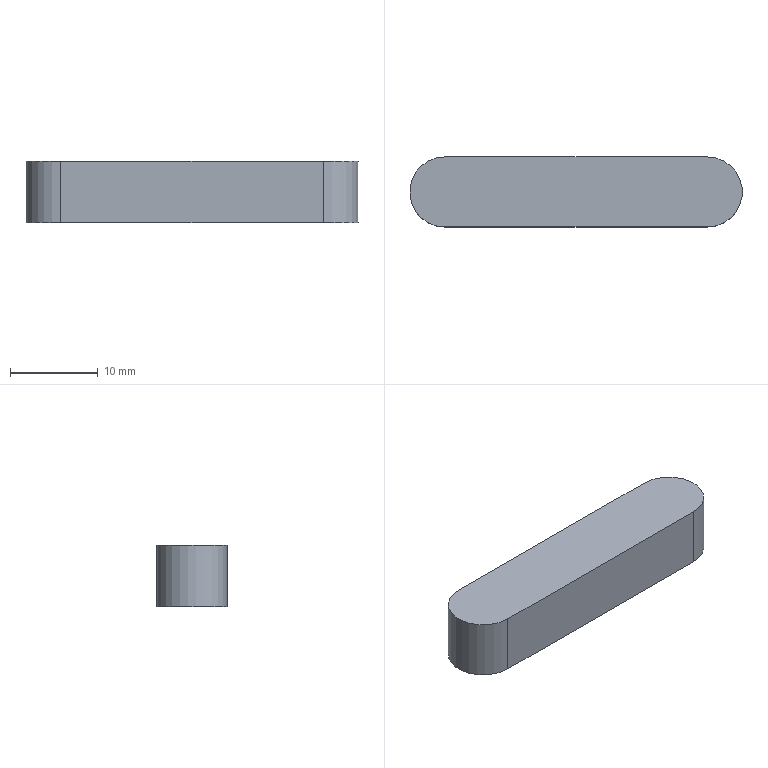Part | NX | features DATUM_CSYS 2, EXTRUDE 1, SKETCH 1 | 1 solid | 6 faces | box 38 x 8 x 7 mm | volume 2032 mm3 | plane 4 | cylinder 2 | commonest cylinder face diameters 8 x2
STEP:
#1=CARTESIAN_POINT('',(-30.,4.,0.));
#2=VERTEX_POINT('',#1);
#3=CARTESIAN_POINT('',(-30.,-4.,0.));
#4=VERTEX_POINT('',#3);
#5=CARTESIAN_POINT('',(-30.,0.,0.));
#6=DIRECTION('',(0.,0.,1.));
#7=DIRECTION('',(1.,0.,0.));
#8=AXIS2_PLACEMENT_3D('',#5,#6,#7);
#9=CIRCLE('',#8,4.);
#10=EDGE_CURVE('',#2,#4,#9,.T.);
#11=ORIENTED_EDGE('',*,*,#10,.T.);
#12=CARTESIAN_POINT('',(-30.,-4.,7.));
#13=VERTEX_POINT('',#12);
#14=CARTESIAN_POINT('',(-30.,-4.,7.));
#15=DIRECTION('',(0.,0.,-1.));
#16=VECTOR('',#15,1000.);
#17=LINE('',#14,#16);
#18=EDGE_CURVE('',#13,#4,#17,.T.);
#19=ORIENTED_EDGE('',*,*,#18,.F.);
#20=CARTESIAN_POINT('',(-30.,4.,7.));
#21=VERTEX_POINT('',#20);
#22=CARTESIAN_POINT('',(-30.,0.,7.));
#23=DIRECTION('',(0.,0.,1.));
#24=DIRECTION('',(1.,0.,0.));
#25=AXIS2_PLACEMENT_3D('',#22,#23,#24);
#26=CIRCLE('',#25,4.);
#27=EDGE_CURVE('',#21,#13,#26,.T.);
#28=ORIENTED_EDGE('',*,*,#27,.F.);
#29=CARTESIAN_POINT('',(-30.,4.,7.));
#30=DIRECTION('',(0.,0.,-1.));
#31=VECTOR('',#30,1000.);
#32=LINE('',#29,#31);
#33=EDGE_CURVE('',#21,#2,#32,.T.);
#34=ORIENTED_EDGE('',*,*,#33,.T.);
#35=EDGE_LOOP('',(#11,#19,#28,#34));
#36=FACE_BOUND('',#35,.T.);
#37=CARTESIAN_POINT('',(-30.,0.,7.));
#38=DIRECTION('',(0.,0.,-1.));
#39=DIRECTION('',(-1.,0.,0.));
#40=AXIS2_PLACEMENT_3D('',#37,#38,#39);
#41=CYLINDRICAL_SURFACE('',#40,4.);
#42=ADVANCED_FACE('',(#36),#41,.T.);
#43=CARTESIAN_POINT('',(0.,-4.,0.));
#44=VERTEX_POINT('',#43);
#45=CARTESIAN_POINT('',(-30.,-4.,0.));
#46=DIRECTION('',(1.,0.,0.));
#47=VECTOR('',#46,1000.);
#48=LINE('',#45,#47);
#49=EDGE_CURVE('',#4,#44,#48,.T.);
#50=ORIENTED_EDGE('',*,*,#49,.T.);
#51=CARTESIAN_POINT('',(0.,-4.,7.));
#52=VERTEX_POINT('',#51);
#53=CARTESIAN_POINT('',(0.,-4.,7.));
#54=DIRECTION('',(0.,0.,-1.));
#55=VECTOR('',#54,1000.);
#56=LINE('',#53,#55);
#57=EDGE_CURVE('',#52,#44,#56,.T.);
#58=ORIENTED_EDGE('',*,*,#57,.F.);
#59=CARTESIAN_POINT('',(-30.,-4.,7.));
#60=DIRECTION('',(1.,0.,0.));
#61=VECTOR('',#60,1000.);
#62=LINE('',#59,#61);
#63=EDGE_CURVE('',#13,#52,#62,.T.);
#64=ORIENTED_EDGE('',*,*,#63,.F.);
#65=ORIENTED_EDGE('',*,*,#18,.T.);
#66=EDGE_LOOP('',(#50,#58,#64,#65));
#67=FACE_BOUND('',#66,.T.);
#68=CARTESIAN_POINT('',(-30.,-4.,7.));
#69=DIRECTION('',(0.,1.,0.));
#70=DIRECTION('',(-1.,0.,0.));
#71=AXIS2_PLACEMENT_3D('',#68,#69,#70);
#72=PLANE('',#71);
#73=ADVANCED_FACE('',(#67),#72,.F.);
#74=CARTESIAN_POINT('',(0.,4.,0.));
#75=VERTEX_POINT('',#74);
#76=CARTESIAN_POINT('',(0.,0.,0.));
#77=DIRECTION('',(0.,0.,1.));
#78=DIRECTION('',(1.,0.,0.));
#79=AXIS2_PLACEMENT_3D('',#76,#77,#78);
#80=CIRCLE('',#79,4.);
#81=EDGE_CURVE('',#44,#75,#80,.T.);
#82=ORIENTED_EDGE('',*,*,#81,.T.);
#83=CARTESIAN_POINT('',(0.,4.,7.));
#84=VERTEX_POINT('',#83);
#85=CARTESIAN_POINT('',(0.,4.,7.));
#86=DIRECTION('',(0.,0.,-1.));
#87=VECTOR('',#86,1000.);
#88=LINE('',#85,#87);
#89=EDGE_CURVE('',#84,#75,#88,.T.);
#90=ORIENTED_EDGE('',*,*,#89,.F.);
#91=CARTESIAN_POINT('',(0.,0.,7.));
#92=DIRECTION('',(0.,0.,1.));
#93=DIRECTION('',(1.,0.,0.));
#94=AXIS2_PLACEMENT_3D('',#91,#92,#93);
#95=CIRCLE('',#94,4.);
#96=EDGE_CURVE('',#52,#84,#95,.T.);
#97=ORIENTED_EDGE('',*,*,#96,.F.);
#98=ORIENTED_EDGE('',*,*,#57,.T.);
#99=EDGE_LOOP('',(#82,#90,#97,#98));
#100=FACE_BOUND('',#99,.T.);
#101=CARTESIAN_POINT('',(0.,0.,7.));
#102=DIRECTION('',(0.,0.,-1.));
#103=DIRECTION('',(-1.,0.,0.));
#104=AXIS2_PLACEMENT_3D('',#101,#102,#103);
#105=CYLINDRICAL_SURFACE('',#104,4.);
#106=ADVANCED_FACE('',(#100),#105,.T.);
#107=CARTESIAN_POINT('',(0.,4.,0.));
#108=DIRECTION('',(-1.,0.,0.));
#109=VECTOR('',#108,1000.);
#110=LINE('',#107,#109);
#111=EDGE_CURVE('',#75,#2,#110,.T.);
#112=ORIENTED_EDGE('',*,*,#111,.T.);
#113=ORIENTED_EDGE('',*,*,#33,.F.);
#114=CARTESIAN_POINT('',(0.,4.,7.));
#115=DIRECTION('',(-1.,0.,0.));
#116=VECTOR('',#115,1000.);
#117=LINE('',#114,#116);
#118=EDGE_CURVE('',#84,#21,#117,.T.);
#119=ORIENTED_EDGE('',*,*,#118,.F.);
#120=ORIENTED_EDGE('',*,*,#89,.T.);
#121=EDGE_LOOP('',(#112,#113,#119,#120));
#122=FACE_BOUND('',#121,.T.);
#123=CARTESIAN_POINT('',(0.,4.,7.));
#124=DIRECTION('',(0.,-1.,0.));
#125=DIRECTION('',(1.,0.,0.));
#126=AXIS2_PLACEMENT_3D('',#123,#124,#125);
#127=PLANE('',#126);
#128=ADVANCED_FACE('',(#122),#127,.F.);
#129=ORIENTED_EDGE('',*,*,#27,.T.);
#130=ORIENTED_EDGE('',*,*,#63,.T.);
#131=ORIENTED_EDGE('',*,*,#96,.T.);
#132=ORIENTED_EDGE('',*,*,#118,.T.);
#133=EDGE_LOOP('',(#129,#130,#131,#132));
#134=FACE_BOUND('',#133,.T.);
#135=CARTESIAN_POINT('',(-30.,0.,7.));
#136=DIRECTION('',(0.,0.,1.));
#137=DIRECTION('',(1.,0.,0.));
#138=AXIS2_PLACEMENT_3D('',#135,#136,#137);
#139=PLANE('',#138);
#140=ADVANCED_FACE('',(#134),#139,.T.);
#141=ORIENTED_EDGE('',*,*,#10,.F.);
#142=ORIENTED_EDGE('',*,*,#111,.F.);
#143=ORIENTED_EDGE('',*,*,#81,.F.);
#144=ORIENTED_EDGE('',*,*,#49,.F.);
#145=EDGE_LOOP('',(#141,#142,#143,#144));
#146=FACE_BOUND('',#145,.T.);
#147=CARTESIAN_POINT('',(-30.,0.,0.));
#148=DIRECTION('',(0.,0.,1.));
#149=DIRECTION('',(1.,0.,0.));
#150=AXIS2_PLACEMENT_3D('',#147,#148,#149);
#151=PLANE('',#150);
#152=ADVANCED_FACE('',(#146),#151,.F.);
#153=CLOSED_SHELL('',(#42,#73,#106,#128,#140,#152));
#154=MANIFOLD_SOLID_BREP('',#153);
#155=(LENGTH_UNIT()NAMED_UNIT(*)SI_UNIT(.MILLI.,.METRE.));
#156=UNCERTAINTY_MEASURE_WITH_UNIT(LENGTH_MEASURE(0.00001),#155,'','');
#157=(NAMED_UNIT(*)PLANE_ANGLE_UNIT()SI_UNIT($,.RADIAN.));
#158=(NAMED_UNIT(*)SI_UNIT($,.STERADIAN.)SOLID_ANGLE_UNIT());
#159=(GEOMETRIC_REPRESENTATION_CONTEXT(3)GLOBAL_UNCERTAINTY_ASSIGNED_CONTEXT((#156))GLOBAL_UNIT_ASSIGNED_CONTEXT((#155,#157,#158))REPRESENTATION_CONTEXT('',''));
#160=ADVANCED_BREP_SHAPE_REPRESENTATION('',(#154),#159);